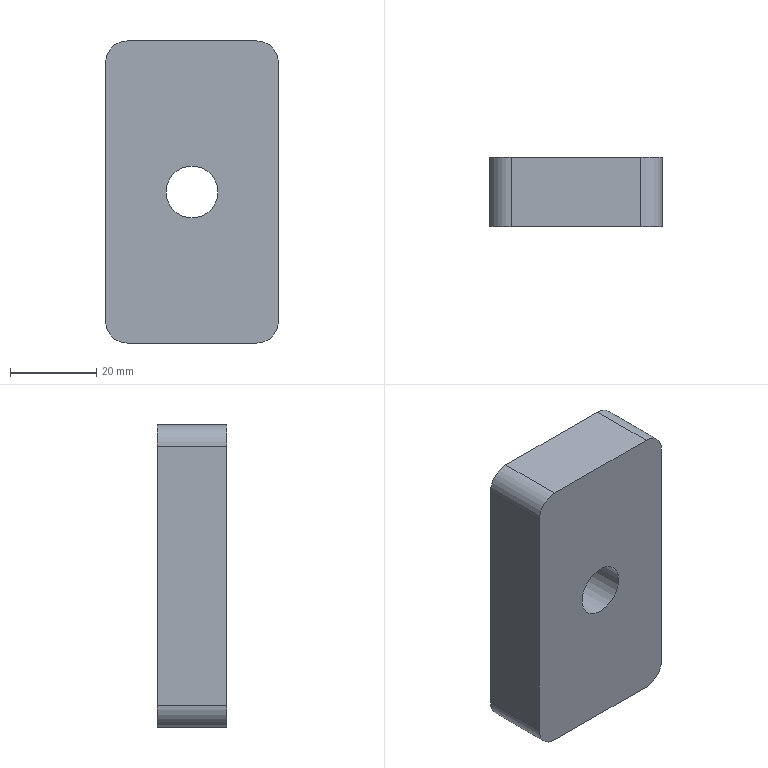Part | STEP file | HL4GZ-1.581.102 (tank fixing seat) | 1 solid | 11 faces | box 40 x 16 x 70 mm | volume 42647 mm3 | plane 6 | cylinder 5 | commonest cylinder face diameters 10 x4 12 x1
STEP:
#1=CARTESIAN_POINT('',(0.,0.,0.));
#2=DIRECTION('',(0.,0.,1.));
#3=DIRECTION('',(1.,0.,0.));
#4=AXIS2_PLACEMENT_3D('',#1,#2,#3);
#5=CARTESIAN_POINT('',(2027.,-666.,-40.));
#6=VERTEX_POINT('',#5);
#7=CARTESIAN_POINT('',(2022.,-666.,-45.));
#8=VERTEX_POINT('',#7);
#9=CARTESIAN_POINT('',(2027.,-666.,-45.));
#10=DIRECTION('',(0.,-1.,0.));
#11=DIRECTION('',(1.,0.,0.));
#12=AXIS2_PLACEMENT_3D('',#9,#10,#11);
#13=CIRCLE('',#12,5.);
#14=CARTESIAN_POINT('',(2027.,-662.,-45.));
#15=DIRECTION('',(0.,-1.,0.));
#16=DIRECTION('',(1.,0.,0.));
#17=AXIS2_PLACEMENT_3D('',#14,#15,#16);
#18=CYLINDRICAL_SURFACE('',#17,5.);
#19=CARTESIAN_POINT('',(0.,4.));
#20=DIRECTION('',(1.,0.));
#21=VECTOR('',#20,1.);
#22=LINE('',#19,#21);
#23=(GEOMETRIC_REPRESENTATION_CONTEXT(2)PARAMETRIC_REPRESENTATION_CONTEXT()REPRESENTATION_CONTEXT('',''));
#24=DEFINITIONAL_REPRESENTATION('',(#22),#23);
#25=PCURVE('',#18,#24);
#26=CARTESIAN_POINT('',(2021.,-666.,-75.));
#27=DIRECTION('',(0.,1.,0.));
#28=DIRECTION('',(1.,0.,0.));
#29=AXIS2_PLACEMENT_3D('',#26,#27,#28);
#30=PLANE('',#29);
#31=CARTESIAN_POINT('',(11.,-30.));
#32=CARTESIAN_POINT('',(11.,-38.66));
#33=CARTESIAN_POINT('',(3.5,-34.33));
#34=CARTESIAN_POINT('',(-4.,-30.));
#35=CARTESIAN_POINT('',(3.5,-25.67));
#36=CARTESIAN_POINT('',(11.,-21.34));
#37=CARTESIAN_POINT('',(11.,-30.));
#38=(BOUNDED_CURVE()B_SPLINE_CURVE(2,(#31,#32,#33,#34,#35,#36,#37),.UNSPECIFIED.,.T.,.F.)B_SPLINE_CURVE_WITH_KNOTS((1,2,2,2,2,1),(-2.094,0.,2.094,4.189,6.283,8.378),.UNSPECIFIED.)CURVE()GEOMETRIC_REPRESENTATION_ITEM()RATIONAL_B_SPLINE_CURVE((1.,0.5,1.,0.5,1.,0.5,1.))REPRESENTATION_ITEM(''));
#39=(GEOMETRIC_REPRESENTATION_CONTEXT(2)PARAMETRIC_REPRESENTATION_CONTEXT()REPRESENTATION_CONTEXT('',''));
#40=DEFINITIONAL_REPRESENTATION('',(#38),#39);
#41=PCURVE('',#30,#40);
#42=SURFACE_CURVE('',#13,(#25,#41),.PCURVE_S1.);
#43=EDGE_CURVE('',#6,#8,#42,.T.);
#44=ORIENTED_EDGE('',*,*,#43,.F.);
#45=CARTESIAN_POINT('',(2027.,-650.,-40.));
#46=VERTEX_POINT('',#45);
#47=CARTESIAN_POINT('',(2027.,-662.,-40.));
#48=DIRECTION('',(0.,-1.,0.));
#49=VECTOR('',#48,1.);
#50=LINE('',#47,#49);
#51=CARTESIAN_POINT('',(1.571,0.));
#52=DIRECTION('',(0.,1.));
#53=VECTOR('',#52,1.);
#54=LINE('',#51,#53);
#55=(GEOMETRIC_REPRESENTATION_CONTEXT(2)PARAMETRIC_REPRESENTATION_CONTEXT()REPRESENTATION_CONTEXT('',''));
#56=DEFINITIONAL_REPRESENTATION('',(#54),#55);
#57=PCURVE('',#18,#56);
#58=CARTESIAN_POINT('',(2062.,-662.,-40.));
#59=DIRECTION('',(0.,0.,-1.));
#60=DIRECTION('',(-1.,0.,0.));
#61=AXIS2_PLACEMENT_3D('',#58,#59,#60);
#62=PLANE('',#61);
#63=CARTESIAN_POINT('',(35.,0.));
#64=DIRECTION('',(0.,-1.));
#65=VECTOR('',#64,1.);
#66=LINE('',#63,#65);
#67=(GEOMETRIC_REPRESENTATION_CONTEXT(2)PARAMETRIC_REPRESENTATION_CONTEXT()REPRESENTATION_CONTEXT('',''));
#68=DEFINITIONAL_REPRESENTATION('',(#66),#67);
#69=PCURVE('',#62,#68);
#70=SURFACE_CURVE('',#50,(#57,#69),.PCURVE_S1.);
#71=EDGE_CURVE('',#46,#6,#70,.T.);
#72=ORIENTED_EDGE('',*,*,#71,.F.);
#73=CARTESIAN_POINT('',(2022.,-650.,-45.));
#74=VERTEX_POINT('',#73);
#75=CARTESIAN_POINT('',(2027.,-650.,-45.));
#76=DIRECTION('',(0.,1.,0.));
#77=DIRECTION('',(1.,0.,0.));
#78=AXIS2_PLACEMENT_3D('',#75,#76,#77);
#79=CIRCLE('',#78,5.);
#80=CARTESIAN_POINT('',(6.283,-12.));
#81=DIRECTION('',(-1.,0.));
#82=VECTOR('',#81,1.);
#83=LINE('',#80,#82);
#84=(GEOMETRIC_REPRESENTATION_CONTEXT(2)PARAMETRIC_REPRESENTATION_CONTEXT()REPRESENTATION_CONTEXT('',''));
#85=DEFINITIONAL_REPRESENTATION('',(#83),#84);
#86=PCURVE('',#18,#85);
#87=CARTESIAN_POINT('',(2021.,-650.,-75.));
#88=DIRECTION('',(0.,1.,0.));
#89=DIRECTION('',(1.,0.,0.));
#90=AXIS2_PLACEMENT_3D('',#87,#88,#89);
#91=PLANE('',#90);
#92=CARTESIAN_POINT('',(6.,-30.));
#93=DIRECTION('',(1.,0.));
#94=AXIS2_PLACEMENT_2D('',#92,#93);
#95=CIRCLE('',#94,5.);
#96=(GEOMETRIC_REPRESENTATION_CONTEXT(2)PARAMETRIC_REPRESENTATION_CONTEXT()REPRESENTATION_CONTEXT('',''));
#97=DEFINITIONAL_REPRESENTATION('',(#95),#96);
#98=PCURVE('',#91,#97);
#99=SURFACE_CURVE('',#79,(#86,#98),.PCURVE_S1.);
#100=EDGE_CURVE('',#74,#46,#99,.T.);
#101=ORIENTED_EDGE('',*,*,#100,.F.);
#102=CARTESIAN_POINT('',(2022.,-662.,-45.));
#103=DIRECTION('',(0.,1.,0.));
#104=VECTOR('',#103,1.);
#105=LINE('',#102,#104);
#106=CARTESIAN_POINT('',(3.142,0.));
#107=DIRECTION('',(0.,-1.));
#108=VECTOR('',#107,1.);
#109=LINE('',#106,#108);
#110=(GEOMETRIC_REPRESENTATION_CONTEXT(2)PARAMETRIC_REPRESENTATION_CONTEXT()REPRESENTATION_CONTEXT('',''));
#111=DEFINITIONAL_REPRESENTATION('',(#109),#110);
#112=PCURVE('',#18,#111);
#113=CARTESIAN_POINT('',(2022.,-662.,-75.));
#114=DIRECTION('',(-1.,0.,0.));
#115=DIRECTION('',(0.,0.,1.));
#116=AXIS2_PLACEMENT_3D('',#113,#114,#115);
#117=PLANE('',#116);
#118=CARTESIAN_POINT('',(30.,0.));
#119=DIRECTION('',(0.,1.));
#120=VECTOR('',#119,1.);
#121=LINE('',#118,#120);
#122=(GEOMETRIC_REPRESENTATION_CONTEXT(2)PARAMETRIC_REPRESENTATION_CONTEXT()REPRESENTATION_CONTEXT('',''));
#123=DEFINITIONAL_REPRESENTATION('',(#121),#122);
#124=PCURVE('',#117,#123);
#125=SURFACE_CURVE('',#105,(#112,#124),.PCURVE_S1.);
#126=EDGE_CURVE('',#8,#74,#125,.T.);
#127=ORIENTED_EDGE('',*,*,#126,.F.);
#128=EDGE_LOOP('',(#44,#72,#101,#127));
#129=FACE_BOUND('',#128,.T.);
#130=ADVANCED_FACE('',(#129),#18,.T.);
#131=CARTESIAN_POINT('',(2022.,-666.,-105.));
#132=VERTEX_POINT('',#131);
#133=CARTESIAN_POINT('',(2027.,-666.,-110.));
#134=VERTEX_POINT('',#133);
#135=CARTESIAN_POINT('',(2027.,-666.,-105.));
#136=DIRECTION('',(0.,-1.,0.));
#137=DIRECTION('',(1.,0.,0.));
#138=AXIS2_PLACEMENT_3D('',#135,#136,#137);
#139=CIRCLE('',#138,5.);
#140=CARTESIAN_POINT('',(2027.,-662.,-105.));
#141=DIRECTION('',(0.,-1.,0.));
#142=DIRECTION('',(1.,0.,0.));
#143=AXIS2_PLACEMENT_3D('',#140,#141,#142);
#144=CYLINDRICAL_SURFACE('',#143,5.);
#145=CARTESIAN_POINT('',(0.,4.));
#146=DIRECTION('',(1.,0.));
#147=VECTOR('',#146,1.);
#148=LINE('',#145,#147);
#149=(GEOMETRIC_REPRESENTATION_CONTEXT(2)PARAMETRIC_REPRESENTATION_CONTEXT()REPRESENTATION_CONTEXT('',''));
#150=DEFINITIONAL_REPRESENTATION('',(#148),#149);
#151=PCURVE('',#144,#150);
#152=CARTESIAN_POINT('',(11.,30.));
#153=CARTESIAN_POINT('',(11.,21.34));
#154=CARTESIAN_POINT('',(3.5,25.67));
#155=CARTESIAN_POINT('',(-4.,30.));
#156=CARTESIAN_POINT('',(3.5,34.33));
#157=CARTESIAN_POINT('',(11.,38.66));
#158=CARTESIAN_POINT('',(11.,30.));
#159=(BOUNDED_CURVE()B_SPLINE_CURVE(2,(#152,#153,#154,#155,#156,#157,#158),.UNSPECIFIED.,.T.,.F.)B_SPLINE_CURVE_WITH_KNOTS((1,2,2,2,2,1),(-2.094,0.,2.094,4.189,6.283,8.378),.UNSPECIFIED.)CURVE()GEOMETRIC_REPRESENTATION_ITEM()RATIONAL_B_SPLINE_CURVE((1.,0.5,1.,0.5,1.,0.5,1.))REPRESENTATION_ITEM(''));
#160=(GEOMETRIC_REPRESENTATION_CONTEXT(2)PARAMETRIC_REPRESENTATION_CONTEXT()REPRESENTATION_CONTEXT('',''));
#161=DEFINITIONAL_REPRESENTATION('',(#159),#160);
#162=PCURVE('',#30,#161);
#163=SURFACE_CURVE('',#139,(#151,#162),.PCURVE_S1.);
#164=EDGE_CURVE('',#132,#134,#163,.T.);
#165=ORIENTED_EDGE('',*,*,#164,.F.);
#166=CARTESIAN_POINT('',(2022.,-650.,-105.));
#167=VERTEX_POINT('',#166);
#168=CARTESIAN_POINT('',(2022.,-662.,-105.));
#169=DIRECTION('',(0.,-1.,0.));
#170=VECTOR('',#169,1.);
#171=LINE('',#168,#170);
#172=CARTESIAN_POINT('',(3.142,0.));
#173=DIRECTION('',(0.,1.));
#174=VECTOR('',#173,1.);
#175=LINE('',#172,#174);
#176=(GEOMETRIC_REPRESENTATION_CONTEXT(2)PARAMETRIC_REPRESENTATION_CONTEXT()REPRESENTATION_CONTEXT('',''));
#177=DEFINITIONAL_REPRESENTATION('',(#175),#176);
#178=PCURVE('',#144,#177);
#179=CARTESIAN_POINT('',(-30.,0.));
#180=DIRECTION('',(0.,-1.));
#181=VECTOR('',#180,1.);
#182=LINE('',#179,#181);
#183=(GEOMETRIC_REPRESENTATION_CONTEXT(2)PARAMETRIC_REPRESENTATION_CONTEXT()REPRESENTATION_CONTEXT('',''));
#184=DEFINITIONAL_REPRESENTATION('',(#182),#183);
#185=PCURVE('',#117,#184);
#186=SURFACE_CURVE('',#171,(#178,#185),.PCURVE_S1.);
#187=EDGE_CURVE('',#167,#132,#186,.T.);
#188=ORIENTED_EDGE('',*,*,#187,.F.);
#189=CARTESIAN_POINT('',(2027.,-650.,-110.));
#190=VERTEX_POINT('',#189);
#191=CARTESIAN_POINT('',(2027.,-650.,-105.));
#192=DIRECTION('',(0.,1.,0.));
#193=DIRECTION('',(1.,0.,0.));
#194=AXIS2_PLACEMENT_3D('',#191,#192,#193);
#195=CIRCLE('',#194,5.);
#196=CARTESIAN_POINT('',(6.283,-12.));
#197=DIRECTION('',(-1.,0.));
#198=VECTOR('',#197,1.);
#199=LINE('',#196,#198);
#200=(GEOMETRIC_REPRESENTATION_CONTEXT(2)PARAMETRIC_REPRESENTATION_CONTEXT()REPRESENTATION_CONTEXT('',''));
#201=DEFINITIONAL_REPRESENTATION('',(#199),#200);
#202=PCURVE('',#144,#201);
#203=CARTESIAN_POINT('',(6.,30.));
#204=DIRECTION('',(1.,0.));
#205=AXIS2_PLACEMENT_2D('',#203,#204);
#206=CIRCLE('',#205,5.);
#207=(GEOMETRIC_REPRESENTATION_CONTEXT(2)PARAMETRIC_REPRESENTATION_CONTEXT()REPRESENTATION_CONTEXT('',''));
#208=DEFINITIONAL_REPRESENTATION('',(#206),#207);
#209=PCURVE('',#91,#208);
#210=SURFACE_CURVE('',#195,(#202,#209),.PCURVE_S1.);
#211=EDGE_CURVE('',#190,#167,#210,.T.);
#212=ORIENTED_EDGE('',*,*,#211,.F.);
#213=CARTESIAN_POINT('',(2027.,-662.,-110.));
#214=DIRECTION('',(0.,1.,0.));
#215=VECTOR('',#214,1.);
#216=LINE('',#213,#215);
#217=CARTESIAN_POINT('',(4.712,0.));
#218=DIRECTION('',(0.,-1.));
#219=VECTOR('',#218,1.);
#220=LINE('',#217,#219);
#221=(GEOMETRIC_REPRESENTATION_CONTEXT(2)PARAMETRIC_REPRESENTATION_CONTEXT()REPRESENTATION_CONTEXT('',''));
#222=DEFINITIONAL_REPRESENTATION('',(#220),#221);
#223=PCURVE('',#144,#222);
#224=CARTESIAN_POINT('',(2062.,-662.,-110.));
#225=DIRECTION('',(0.,0.,1.));
#226=DIRECTION('',(1.,0.,0.));
#227=AXIS2_PLACEMENT_3D('',#224,#225,#226);
#228=PLANE('',#227);
#229=CARTESIAN_POINT('',(-35.,0.));
#230=DIRECTION('',(0.,1.));
#231=VECTOR('',#230,1.);
#232=LINE('',#229,#231);
#233=(GEOMETRIC_REPRESENTATION_CONTEXT(2)PARAMETRIC_REPRESENTATION_CONTEXT()REPRESENTATION_CONTEXT('',''));
#234=DEFINITIONAL_REPRESENTATION('',(#232),#233);
#235=PCURVE('',#228,#234);
#236=SURFACE_CURVE('',#216,(#223,#235),.PCURVE_S1.);
#237=EDGE_CURVE('',#134,#190,#236,.T.);
#238=ORIENTED_EDGE('',*,*,#237,.F.);
#239=EDGE_LOOP('',(#165,#188,#212,#238));
#240=FACE_BOUND('',#239,.T.);
#241=ADVANCED_FACE('',(#240),#144,.T.);
#242=CARTESIAN_POINT('',(2062.,-666.,-45.));
#243=VERTEX_POINT('',#242);
#244=CARTESIAN_POINT('',(2057.,-666.,-40.));
#245=VERTEX_POINT('',#244);
#246=CARTESIAN_POINT('',(2057.,-666.,-45.));
#247=DIRECTION('',(0.,-1.,0.));
#248=DIRECTION('',(1.,0.,0.));
#249=AXIS2_PLACEMENT_3D('',#246,#247,#248);
#250=CIRCLE('',#249,5.);
#251=CARTESIAN_POINT('',(2057.,-662.,-45.));
#252=DIRECTION('',(0.,-1.,0.));
#253=DIRECTION('',(1.,0.,0.));
#254=AXIS2_PLACEMENT_3D('',#251,#252,#253);
#255=CYLINDRICAL_SURFACE('',#254,5.);
#256=CARTESIAN_POINT('',(0.,4.));
#257=DIRECTION('',(1.,0.));
#258=VECTOR('',#257,1.);
#259=LINE('',#256,#258);
#260=(GEOMETRIC_REPRESENTATION_CONTEXT(2)PARAMETRIC_REPRESENTATION_CONTEXT()REPRESENTATION_CONTEXT('',''));
#261=DEFINITIONAL_REPRESENTATION('',(#259),#260);
#262=PCURVE('',#255,#261);
#263=CARTESIAN_POINT('',(41.,-30.));
#264=CARTESIAN_POINT('',(41.,-38.66));
#265=CARTESIAN_POINT('',(33.5,-34.33));
#266=CARTESIAN_POINT('',(26.,-30.));
#267=CARTESIAN_POINT('',(33.5,-25.67));
#268=CARTESIAN_POINT('',(41.,-21.34));
#269=CARTESIAN_POINT('',(41.,-30.));
#270=(BOUNDED_CURVE()B_SPLINE_CURVE(2,(#263,#264,#265,#266,#267,#268,#269),.UNSPECIFIED.,.T.,.F.)B_SPLINE_CURVE_WITH_KNOTS((1,2,2,2,2,1),(-2.094,0.,2.094,4.189,6.283,8.378),.UNSPECIFIED.)CURVE()GEOMETRIC_REPRESENTATION_ITEM()RATIONAL_B_SPLINE_CURVE((1.,0.5,1.,0.5,1.,0.5,1.))REPRESENTATION_ITEM(''));
#271=(GEOMETRIC_REPRESENTATION_CONTEXT(2)PARAMETRIC_REPRESENTATION_CONTEXT()REPRESENTATION_CONTEXT('',''));
#272=DEFINITIONAL_REPRESENTATION('',(#270),#271);
#273=PCURVE('',#30,#272);
#274=SURFACE_CURVE('',#250,(#262,#273),.PCURVE_S1.);
#275=EDGE_CURVE('',#243,#245,#274,.T.);
#276=ORIENTED_EDGE('',*,*,#275,.F.);
#277=CARTESIAN_POINT('',(2062.,-650.,-45.));
#278=VERTEX_POINT('',#277);
#279=CARTESIAN_POINT('',(2062.,-662.,-45.));
#280=DIRECTION('',(0.,-1.,0.));
#281=VECTOR('',#280,1.);
#282=LINE('',#279,#281);
#283=CARTESIAN_POINT('',(0.,0.));
#284=DIRECTION('',(0.,1.));
#285=VECTOR('',#284,1.);
#286=LINE('',#283,#285);
#287=(GEOMETRIC_REPRESENTATION_CONTEXT(2)PARAMETRIC_REPRESENTATION_CONTEXT()REPRESENTATION_CONTEXT('',''));
#288=DEFINITIONAL_REPRESENTATION('',(#286),#287);
#289=PCURVE('',#255,#288);
#290=CARTESIAN_POINT('',(2062.,-662.,-75.));
#291=DIRECTION('',(1.,0.,0.));
#292=DIRECTION('',(0.,0.,-1.));
#293=AXIS2_PLACEMENT_3D('',#290,#291,#292);
#294=PLANE('',#293);
#295=CARTESIAN_POINT('',(-30.,0.));
#296=DIRECTION('',(0.,-1.));
#297=VECTOR('',#296,1.);
#298=LINE('',#295,#297);
#299=(GEOMETRIC_REPRESENTATION_CONTEXT(2)PARAMETRIC_REPRESENTATION_CONTEXT()REPRESENTATION_CONTEXT('',''));
#300=DEFINITIONAL_REPRESENTATION('',(#298),#299);
#301=PCURVE('',#294,#300);
#302=SURFACE_CURVE('',#282,(#289,#301),.PCURVE_S1.);
#303=EDGE_CURVE('',#278,#243,#302,.T.);
#304=ORIENTED_EDGE('',*,*,#303,.F.);
#305=CARTESIAN_POINT('',(2057.,-650.,-40.));
#306=VERTEX_POINT('',#305);
#307=CARTESIAN_POINT('',(2057.,-650.,-45.));
#308=DIRECTION('',(0.,1.,0.));
#309=DIRECTION('',(1.,0.,0.));
#310=AXIS2_PLACEMENT_3D('',#307,#308,#309);
#311=CIRCLE('',#310,5.);
#312=CARTESIAN_POINT('',(6.283,-12.));
#313=DIRECTION('',(-1.,0.));
#314=VECTOR('',#313,1.);
#315=LINE('',#312,#314);
#316=(GEOMETRIC_REPRESENTATION_CONTEXT(2)PARAMETRIC_REPRESENTATION_CONTEXT()REPRESENTATION_CONTEXT('',''));
#317=DEFINITIONAL_REPRESENTATION('',(#315),#316);
#318=PCURVE('',#255,#317);
#319=CARTESIAN_POINT('',(36.,-30.));
#320=DIRECTION('',(1.,0.));
#321=AXIS2_PLACEMENT_2D('',#319,#320);
#322=CIRCLE('',#321,5.);
#323=(GEOMETRIC_REPRESENTATION_CONTEXT(2)PARAMETRIC_REPRESENTATION_CONTEXT()REPRESENTATION_CONTEXT('',''));
#324=DEFINITIONAL_REPRESENTATION('',(#322),#323);
#325=PCURVE('',#91,#324);
#326=SURFACE_CURVE('',#311,(#318,#325),.PCURVE_S1.);
#327=EDGE_CURVE('',#306,#278,#326,.T.);
#328=ORIENTED_EDGE('',*,*,#327,.F.);
#329=CARTESIAN_POINT('',(2057.,-662.,-40.));
#330=DIRECTION('',(0.,1.,0.));
#331=VECTOR('',#330,1.);
#332=LINE('',#329,#331);
#333=CARTESIAN_POINT('',(1.571,0.));
#334=DIRECTION('',(0.,-1.));
#335=VECTOR('',#334,1.);
#336=LINE('',#333,#335);
#337=(GEOMETRIC_REPRESENTATION_CONTEXT(2)PARAMETRIC_REPRESENTATION_CONTEXT()REPRESENTATION_CONTEXT('',''));
#338=DEFINITIONAL_REPRESENTATION('',(#336),#337);
#339=PCURVE('',#255,#338);
#340=CARTESIAN_POINT('',(5.,0.));
#341=DIRECTION('',(0.,1.));
#342=VECTOR('',#341,1.);
#343=LINE('',#340,#342);
#344=(GEOMETRIC_REPRESENTATION_CONTEXT(2)PARAMETRIC_REPRESENTATION_CONTEXT()REPRESENTATION_CONTEXT('',''));
#345=DEFINITIONAL_REPRESENTATION('',(#343),#344);
#346=PCURVE('',#62,#345);
#347=SURFACE_CURVE('',#332,(#339,#346),.PCURVE_S1.);
#348=EDGE_CURVE('',#245,#306,#347,.T.);
#349=ORIENTED_EDGE('',*,*,#348,.F.);
#350=EDGE_LOOP('',(#276,#304,#328,#349));
#351=FACE_BOUND('',#350,.T.);
#352=ADVANCED_FACE('',(#351),#255,.T.);
#353=CARTESIAN_POINT('',(2057.,-666.,-110.));
#354=VERTEX_POINT('',#353);
#355=CARTESIAN_POINT('',(2062.,-666.,-105.));
#356=VERTEX_POINT('',#355);
#357=CARTESIAN_POINT('',(2057.,-666.,-105.));
#358=DIRECTION('',(0.,-1.,0.));
#359=DIRECTION('',(1.,0.,0.));
#360=AXIS2_PLACEMENT_3D('',#357,#358,#359);
#361=CIRCLE('',#360,5.);
#362=CARTESIAN_POINT('',(2057.,-662.,-105.));
#363=DIRECTION('',(0.,1.,0.));
#364=DIRECTION('',(-1.,0.,0.));
#365=AXIS2_PLACEMENT_3D('',#362,#363,#364);
#366=CYLINDRICAL_SURFACE('',#365,5.);
#367=CARTESIAN_POINT('',(9.425,-4.));
#368=DIRECTION('',(-1.,0.));
#369=VECTOR('',#368,1.);
#370=LINE('',#367,#369);
#371=(GEOMETRIC_REPRESENTATION_CONTEXT(2)PARAMETRIC_REPRESENTATION_CONTEXT()REPRESENTATION_CONTEXT('',''));
#372=DEFINITIONAL_REPRESENTATION('',(#370),#371);
#373=PCURVE('',#366,#372);
#374=CARTESIAN_POINT('',(41.,30.));
#375=CARTESIAN_POINT('',(41.,21.34));
#376=CARTESIAN_POINT('',(33.5,25.67));
#377=CARTESIAN_POINT('',(26.,30.));
#378=CARTESIAN_POINT('',(33.5,34.33));
#379=CARTESIAN_POINT('',(41.,38.66));
#380=CARTESIAN_POINT('',(41.,30.));
#381=(BOUNDED_CURVE()B_SPLINE_CURVE(2,(#374,#375,#376,#377,#378,#379,#380),.UNSPECIFIED.,.T.,.F.)B_SPLINE_CURVE_WITH_KNOTS((1,2,2,2,2,1),(-2.094,0.,2.094,4.189,6.283,8.378),.UNSPECIFIED.)CURVE()GEOMETRIC_REPRESENTATION_ITEM()RATIONAL_B_SPLINE_CURVE((1.,0.5,1.,0.5,1.,0.5,1.))REPRESENTATION_ITEM(''));
#382=(GEOMETRIC_REPRESENTATION_CONTEXT(2)PARAMETRIC_REPRESENTATION_CONTEXT()REPRESENTATION_CONTEXT('',''));
#383=DEFINITIONAL_REPRESENTATION('',(#381),#382);
#384=PCURVE('',#30,#383);
#385=SURFACE_CURVE('',#361,(#373,#384),.PCURVE_S1.);
#386=EDGE_CURVE('',#354,#356,#385,.T.);
#387=ORIENTED_EDGE('',*,*,#386,.F.);
#388=CARTESIAN_POINT('',(2057.,-650.,-110.));
#389=VERTEX_POINT('',#388);
#390=CARTESIAN_POINT('',(2057.,-662.,-110.));
#391=DIRECTION('',(0.,-1.,0.));
#392=VECTOR('',#391,1.);
#393=LINE('',#390,#392);
#394=CARTESIAN_POINT('',(4.712,0.));
#395=DIRECTION('',(0.,-1.));
#396=VECTOR('',#395,1.);
#397=LINE('',#394,#396);
#398=(GEOMETRIC_REPRESENTATION_CONTEXT(2)PARAMETRIC_REPRESENTATION_CONTEXT()REPRESENTATION_CONTEXT('',''));
#399=DEFINITIONAL_REPRESENTATION('',(#397),#398);
#400=PCURVE('',#366,#399);
#401=CARTESIAN_POINT('',(-5.,0.));
#402=DIRECTION('',(0.,-1.));
#403=VECTOR('',#402,1.);
#404=LINE('',#401,#403);
#405=(GEOMETRIC_REPRESENTATION_CONTEXT(2)PARAMETRIC_REPRESENTATION_CONTEXT()REPRESENTATION_CONTEXT('',''));
#406=DEFINITIONAL_REPRESENTATION('',(#404),#405);
#407=PCURVE('',#228,#406);
#408=SURFACE_CURVE('',#393,(#400,#407),.PCURVE_S1.);
#409=EDGE_CURVE('',#389,#354,#408,.T.);
#410=ORIENTED_EDGE('',*,*,#409,.F.);
#411=CARTESIAN_POINT('',(2062.,-650.,-105.));
#412=VERTEX_POINT('',#411);
#413=CARTESIAN_POINT('',(2057.,-650.,-105.));
#414=DIRECTION('',(0.,1.,0.));
#415=DIRECTION('',(1.,0.,0.));
#416=AXIS2_PLACEMENT_3D('',#413,#414,#415);
#417=CIRCLE('',#416,5.);
#418=CARTESIAN_POINT('',(3.142,12.));
#419=DIRECTION('',(1.,0.));
#420=VECTOR('',#419,1.);
#421=LINE('',#418,#420);
#422=(GEOMETRIC_REPRESENTATION_CONTEXT(2)PARAMETRIC_REPRESENTATION_CONTEXT()REPRESENTATION_CONTEXT('',''));
#423=DEFINITIONAL_REPRESENTATION('',(#421),#422);
#424=PCURVE('',#366,#423);
#425=CARTESIAN_POINT('',(36.,30.));
#426=DIRECTION('',(1.,0.));
#427=AXIS2_PLACEMENT_2D('',#425,#426);
#428=CIRCLE('',#427,5.);
#429=(GEOMETRIC_REPRESENTATION_CONTEXT(2)PARAMETRIC_REPRESENTATION_CONTEXT()REPRESENTATION_CONTEXT('',''));
#430=DEFINITIONAL_REPRESENTATION('',(#428),#429);
#431=PCURVE('',#91,#430);
#432=SURFACE_CURVE('',#417,(#424,#431),.PCURVE_S1.);
#433=EDGE_CURVE('',#412,#389,#432,.T.);
#434=ORIENTED_EDGE('',*,*,#433,.F.);
#435=CARTESIAN_POINT('',(2062.,-662.,-105.));
#436=DIRECTION('',(0.,1.,0.));
#437=VECTOR('',#436,1.);
#438=LINE('',#435,#437);
#439=CARTESIAN_POINT('',(3.142,0.));
#440=DIRECTION('',(0.,1.));
#441=VECTOR('',#440,1.);
#442=LINE('',#439,#441);
#443=(GEOMETRIC_REPRESENTATION_CONTEXT(2)PARAMETRIC_REPRESENTATION_CONTEXT()REPRESENTATION_CONTEXT('',''));
#444=DEFINITIONAL_REPRESENTATION('',(#442),#443);
#445=PCURVE('',#366,#444);
#446=CARTESIAN_POINT('',(30.,0.));
#447=DIRECTION('',(0.,1.));
#448=VECTOR('',#447,1.);
#449=LINE('',#446,#448);
#450=(GEOMETRIC_REPRESENTATION_CONTEXT(2)PARAMETRIC_REPRESENTATION_CONTEXT()REPRESENTATION_CONTEXT('',''));
#451=DEFINITIONAL_REPRESENTATION('',(#449),#450);
#452=PCURVE('',#294,#451);
#453=SURFACE_CURVE('',#438,(#445,#452),.PCURVE_S1.);
#454=EDGE_CURVE('',#356,#412,#453,.T.);
#455=ORIENTED_EDGE('',*,*,#454,.F.);
#456=EDGE_LOOP('',(#387,#410,#434,#455));
#457=FACE_BOUND('',#456,.T.);
#458=ADVANCED_FACE('',(#457),#366,.T.);
#459=CARTESIAN_POINT('',(2048.,-666.,-75.));
#460=VERTEX_POINT('',#459);
#461=CARTESIAN_POINT('',(2042.,-666.,-75.));
#462=DIRECTION('',(0.,-1.,0.));
#463=DIRECTION('',(1.,0.,0.));
#464=AXIS2_PLACEMENT_3D('',#461,#462,#463);
#465=CIRCLE('',#464,6.);
#466=CARTESIAN_POINT('',(27.,0.));
#467=CARTESIAN_POINT('',(27.,-10.392));
#468=CARTESIAN_POINT('',(18.,-5.196));
#469=CARTESIAN_POINT('',(9.,0.));
#470=CARTESIAN_POINT('',(18.,5.196));
#471=CARTESIAN_POINT('',(27.,10.392));
#472=CARTESIAN_POINT('',(27.,0.));
#473=(BOUNDED_CURVE()B_SPLINE_CURVE(2,(#466,#467,#468,#469,#470,#471,#472),.UNSPECIFIED.,.T.,.F.)B_SPLINE_CURVE_WITH_KNOTS((1,2,2,2,2,1),(-2.094,0.,2.094,4.189,6.283,8.378),.UNSPECIFIED.)CURVE()GEOMETRIC_REPRESENTATION_ITEM()RATIONAL_B_SPLINE_CURVE((1.,0.5,1.,0.5,1.,0.5,1.))REPRESENTATION_ITEM(''));
#474=(GEOMETRIC_REPRESENTATION_CONTEXT(2)PARAMETRIC_REPRESENTATION_CONTEXT()REPRESENTATION_CONTEXT('',''));
#475=DEFINITIONAL_REPRESENTATION('',(#473),#474);
#476=PCURVE('',#30,#475);
#477=CARTESIAN_POINT('',(2042.,-662.,-75.));
#478=DIRECTION('',(0.,-1.,0.));
#479=DIRECTION('',(1.,0.,0.));
#480=AXIS2_PLACEMENT_3D('',#477,#478,#479);
#481=CYLINDRICAL_SURFACE('',#480,6.);
#482=CARTESIAN_POINT('',(0.,4.));
#483=DIRECTION('',(1.,0.));
#484=VECTOR('',#483,1.);
#485=LINE('',#482,#484);
#486=(GEOMETRIC_REPRESENTATION_CONTEXT(2)PARAMETRIC_REPRESENTATION_CONTEXT()REPRESENTATION_CONTEXT('',''));
#487=DEFINITIONAL_REPRESENTATION('',(#485),#486);
#488=PCURVE('',#481,#487);
#489=SURFACE_CURVE('',#465,(#476,#488),.PCURVE_S1.);
#490=EDGE_CURVE('',#460,#460,#489,.T.);
#491=ORIENTED_EDGE('',*,*,#490,.F.);
#492=EDGE_LOOP('',(#491));
#493=FACE_BOUND('',#492,.T.);
#494=CARTESIAN_POINT('',(2022.,-666.,-75.));
#495=DIRECTION('',(0.,0.,1.));
#496=VECTOR('',#495,1.);
#497=LINE('',#494,#496);
#498=CARTESIAN_POINT('',(1.,0.));
#499=DIRECTION('',(0.,-1.));
#500=VECTOR('',#499,1.);
#501=LINE('',#498,#500);
#502=(GEOMETRIC_REPRESENTATION_CONTEXT(2)PARAMETRIC_REPRESENTATION_CONTEXT()REPRESENTATION_CONTEXT('',''));
#503=DEFINITIONAL_REPRESENTATION('',(#501),#502);
#504=PCURVE('',#30,#503);
#505=CARTESIAN_POINT('',(0.,-4.));
#506=DIRECTION('',(1.,0.));
#507=VECTOR('',#506,1.);
#508=LINE('',#505,#507);
#509=(GEOMETRIC_REPRESENTATION_CONTEXT(2)PARAMETRIC_REPRESENTATION_CONTEXT()REPRESENTATION_CONTEXT('',''));
#510=DEFINITIONAL_REPRESENTATION('',(#508),#509);
#511=PCURVE('',#117,#510);
#512=SURFACE_CURVE('',#497,(#504,#511),.PCURVE_S1.);
#513=EDGE_CURVE('',#132,#8,#512,.T.);
#514=ORIENTED_EDGE('',*,*,#513,.F.);
#515=ORIENTED_EDGE('',*,*,#164,.T.);
#516=CARTESIAN_POINT('',(2062.,-666.,-110.));
#517=DIRECTION('',(1.,0.,0.));
#518=VECTOR('',#517,1.);
#519=LINE('',#516,#518);
#520=CARTESIAN_POINT('',(41.,35.));
#521=DIRECTION('',(1.,0.));
#522=VECTOR('',#521,1.);
#523=LINE('',#520,#522);
#524=(GEOMETRIC_REPRESENTATION_CONTEXT(2)PARAMETRIC_REPRESENTATION_CONTEXT()REPRESENTATION_CONTEXT('',''));
#525=DEFINITIONAL_REPRESENTATION('',(#523),#524);
#526=PCURVE('',#30,#525);
#527=CARTESIAN_POINT('',(0.,-4.));
#528=DIRECTION('',(1.,0.));
#529=VECTOR('',#528,1.);
#530=LINE('',#527,#529);
#531=(GEOMETRIC_REPRESENTATION_CONTEXT(2)PARAMETRIC_REPRESENTATION_CONTEXT()REPRESENTATION_CONTEXT('',''));
#532=DEFINITIONAL_REPRESENTATION('',(#530),#531);
#533=PCURVE('',#228,#532);
#534=SURFACE_CURVE('',#519,(#526,#533),.PCURVE_S1.);
#535=EDGE_CURVE('',#134,#354,#534,.T.);
#536=ORIENTED_EDGE('',*,*,#535,.T.);
#537=ORIENTED_EDGE('',*,*,#386,.T.);
#538=CARTESIAN_POINT('',(2062.,-666.,-75.));
#539=DIRECTION('',(0.,0.,-1.));
#540=VECTOR('',#539,1.);
#541=LINE('',#538,#540);
#542=CARTESIAN_POINT('',(41.,0.));
#543=DIRECTION('',(0.,1.));
#544=VECTOR('',#543,1.);
#545=LINE('',#542,#544);
#546=(GEOMETRIC_REPRESENTATION_CONTEXT(2)PARAMETRIC_REPRESENTATION_CONTEXT()REPRESENTATION_CONTEXT('',''));
#547=DEFINITIONAL_REPRESENTATION('',(#545),#546);
#548=PCURVE('',#30,#547);
#549=CARTESIAN_POINT('',(0.,-4.));
#550=DIRECTION('',(1.,0.));
#551=VECTOR('',#550,1.);
#552=LINE('',#549,#551);
#553=(GEOMETRIC_REPRESENTATION_CONTEXT(2)PARAMETRIC_REPRESENTATION_CONTEXT()REPRESENTATION_CONTEXT('',''));
#554=DEFINITIONAL_REPRESENTATION('',(#552),#553);
#555=PCURVE('',#294,#554);
#556=SURFACE_CURVE('',#541,(#548,#555),.PCURVE_S1.);
#557=EDGE_CURVE('',#243,#356,#556,.T.);
#558=ORIENTED_EDGE('',*,*,#557,.F.);
#559=ORIENTED_EDGE('',*,*,#275,.T.);
#560=CARTESIAN_POINT('',(2062.,-666.,-40.));
#561=DIRECTION('',(-1.,0.,0.));
#562=VECTOR('',#561,1.);
#563=LINE('',#560,#562);
#564=CARTESIAN_POINT('',(41.,-35.));
#565=DIRECTION('',(-1.,0.));
#566=VECTOR('',#565,1.);
#567=LINE('',#564,#566);
#568=(GEOMETRIC_REPRESENTATION_CONTEXT(2)PARAMETRIC_REPRESENTATION_CONTEXT()REPRESENTATION_CONTEXT('',''));
#569=DEFINITIONAL_REPRESENTATION('',(#567),#568);
#570=PCURVE('',#30,#569);
#571=CARTESIAN_POINT('',(0.,-4.));
#572=DIRECTION('',(1.,0.));
#573=VECTOR('',#572,1.);
#574=LINE('',#571,#573);
#575=(GEOMETRIC_REPRESENTATION_CONTEXT(2)PARAMETRIC_REPRESENTATION_CONTEXT()REPRESENTATION_CONTEXT('',''));
#576=DEFINITIONAL_REPRESENTATION('',(#574),#575);
#577=PCURVE('',#62,#576);
#578=SURFACE_CURVE('',#563,(#570,#577),.PCURVE_S1.);
#579=EDGE_CURVE('',#245,#6,#578,.T.);
#580=ORIENTED_EDGE('',*,*,#579,.T.);
#581=ORIENTED_EDGE('',*,*,#43,.T.);
#582=EDGE_LOOP('',(#514,#515,#536,#537,#558,#559,#580,#581));
#583=FACE_BOUND('',#582,.T.);
#584=ADVANCED_FACE('',(#493,#583),#30,.F.);
#585=CARTESIAN_POINT('',(2048.,-650.,-75.));
#586=VERTEX_POINT('',#585);
#587=CARTESIAN_POINT('',(2042.,-650.,-75.));
#588=DIRECTION('',(0.,-1.,0.));
#589=DIRECTION('',(1.,0.,0.));
#590=AXIS2_PLACEMENT_3D('',#587,#588,#589);
#591=CIRCLE('',#590,6.);
#592=CARTESIAN_POINT('',(27.,0.));
#593=CARTESIAN_POINT('',(27.,-10.392));
#594=CARTESIAN_POINT('',(18.,-5.196));
#595=CARTESIAN_POINT('',(9.,0.));
#596=CARTESIAN_POINT('',(18.,5.196));
#597=CARTESIAN_POINT('',(27.,10.392));
#598=CARTESIAN_POINT('',(27.,0.));
#599=(BOUNDED_CURVE()B_SPLINE_CURVE(2,(#592,#593,#594,#595,#596,#597,#598),.UNSPECIFIED.,.T.,.F.)B_SPLINE_CURVE_WITH_KNOTS((1,2,2,2,2,1),(-2.094,0.,2.094,4.189,6.283,8.378),.UNSPECIFIED.)CURVE()GEOMETRIC_REPRESENTATION_ITEM()RATIONAL_B_SPLINE_CURVE((1.,0.5,1.,0.5,1.,0.5,1.))REPRESENTATION_ITEM(''));
#600=(GEOMETRIC_REPRESENTATION_CONTEXT(2)PARAMETRIC_REPRESENTATION_CONTEXT()REPRESENTATION_CONTEXT('',''));
#601=DEFINITIONAL_REPRESENTATION('',(#599),#600);
#602=PCURVE('',#91,#601);
#603=CARTESIAN_POINT('',(0.,-12.));
#604=DIRECTION('',(1.,0.));
#605=VECTOR('',#604,1.);
#606=LINE('',#603,#605);
#607=(GEOMETRIC_REPRESENTATION_CONTEXT(2)PARAMETRIC_REPRESENTATION_CONTEXT()REPRESENTATION_CONTEXT('',''));
#608=DEFINITIONAL_REPRESENTATION('',(#606),#607);
#609=PCURVE('',#481,#608);
#610=SURFACE_CURVE('',#591,(#602,#609),.PCURVE_S1.);
#611=EDGE_CURVE('',#586,#586,#610,.T.);
#612=ORIENTED_EDGE('',*,*,#611,.T.);
#613=EDGE_LOOP('',(#612));
#614=FACE_BOUND('',#613,.T.);
#615=CARTESIAN_POINT('',(2021.,-650.,-40.));
#616=DIRECTION('',(-1.,0.,0.));
#617=VECTOR('',#616,1.);
#618=LINE('',#615,#617);
#619=CARTESIAN_POINT('',(0.,-35.));
#620=DIRECTION('',(-1.,0.));
#621=VECTOR('',#620,1.);
#622=LINE('',#619,#621);
#623=(GEOMETRIC_REPRESENTATION_CONTEXT(2)PARAMETRIC_REPRESENTATION_CONTEXT()REPRESENTATION_CONTEXT('',''));
#624=DEFINITIONAL_REPRESENTATION('',(#622),#623);
#625=PCURVE('',#91,#624);
#626=CARTESIAN_POINT('',(41.,12.));
#627=DIRECTION('',(1.,0.));
#628=VECTOR('',#627,1.);
#629=LINE('',#626,#628);
#630=(GEOMETRIC_REPRESENTATION_CONTEXT(2)PARAMETRIC_REPRESENTATION_CONTEXT()REPRESENTATION_CONTEXT('',''));
#631=DEFINITIONAL_REPRESENTATION('',(#629),#630);
#632=PCURVE('',#62,#631);
#633=SURFACE_CURVE('',#618,(#625,#632),.PCURVE_S1.);
#634=EDGE_CURVE('',#306,#46,#633,.T.);
#635=ORIENTED_EDGE('',*,*,#634,.F.);
#636=ORIENTED_EDGE('',*,*,#327,.T.);
#637=CARTESIAN_POINT('',(2062.,-650.,-75.));
#638=DIRECTION('',(0.,0.,-1.));
#639=VECTOR('',#638,1.);
#640=LINE('',#637,#639);
#641=CARTESIAN_POINT('',(41.,0.));
#642=DIRECTION('',(0.,1.));
#643=VECTOR('',#642,1.);
#644=LINE('',#641,#643);
#645=(GEOMETRIC_REPRESENTATION_CONTEXT(2)PARAMETRIC_REPRESENTATION_CONTEXT()REPRESENTATION_CONTEXT('',''));
#646=DEFINITIONAL_REPRESENTATION('',(#644),#645);
#647=PCURVE('',#91,#646);
#648=CARTESIAN_POINT('',(0.,12.));
#649=DIRECTION('',(1.,0.));
#650=VECTOR('',#649,1.);
#651=LINE('',#648,#650);
#652=(GEOMETRIC_REPRESENTATION_CONTEXT(2)PARAMETRIC_REPRESENTATION_CONTEXT()REPRESENTATION_CONTEXT('',''));
#653=DEFINITIONAL_REPRESENTATION('',(#651),#652);
#654=PCURVE('',#294,#653);
#655=SURFACE_CURVE('',#640,(#647,#654),.PCURVE_S1.);
#656=EDGE_CURVE('',#278,#412,#655,.T.);
#657=ORIENTED_EDGE('',*,*,#656,.T.);
#658=ORIENTED_EDGE('',*,*,#433,.T.);
#659=CARTESIAN_POINT('',(2021.,-650.,-110.));
#660=DIRECTION('',(1.,0.,0.));
#661=VECTOR('',#660,1.);
#662=LINE('',#659,#661);
#663=CARTESIAN_POINT('',(0.,35.));
#664=DIRECTION('',(1.,0.));
#665=VECTOR('',#664,1.);
#666=LINE('',#663,#665);
#667=(GEOMETRIC_REPRESENTATION_CONTEXT(2)PARAMETRIC_REPRESENTATION_CONTEXT()REPRESENTATION_CONTEXT('',''));
#668=DEFINITIONAL_REPRESENTATION('',(#666),#667);
#669=PCURVE('',#91,#668);
#670=CARTESIAN_POINT('',(-41.,12.));
#671=DIRECTION('',(1.,0.));
#672=VECTOR('',#671,1.);
#673=LINE('',#670,#672);
#674=(GEOMETRIC_REPRESENTATION_CONTEXT(2)PARAMETRIC_REPRESENTATION_CONTEXT()REPRESENTATION_CONTEXT('',''));
#675=DEFINITIONAL_REPRESENTATION('',(#673),#674);
#676=PCURVE('',#228,#675);
#677=SURFACE_CURVE('',#662,(#669,#676),.PCURVE_S1.);
#678=EDGE_CURVE('',#190,#389,#677,.T.);
#679=ORIENTED_EDGE('',*,*,#678,.F.);
#680=ORIENTED_EDGE('',*,*,#211,.T.);
#681=CARTESIAN_POINT('',(2022.,-650.,-75.));
#682=DIRECTION('',(0.,0.,1.));
#683=VECTOR('',#682,1.);
#684=LINE('',#681,#683);
#685=CARTESIAN_POINT('',(1.,0.));
#686=DIRECTION('',(0.,-1.));
#687=VECTOR('',#686,1.);
#688=LINE('',#685,#687);
#689=(GEOMETRIC_REPRESENTATION_CONTEXT(2)PARAMETRIC_REPRESENTATION_CONTEXT()REPRESENTATION_CONTEXT('',''));
#690=DEFINITIONAL_REPRESENTATION('',(#688),#689);
#691=PCURVE('',#91,#690);
#692=CARTESIAN_POINT('',(0.,12.));
#693=DIRECTION('',(1.,0.));
#694=VECTOR('',#693,1.);
#695=LINE('',#692,#694);
#696=(GEOMETRIC_REPRESENTATION_CONTEXT(2)PARAMETRIC_REPRESENTATION_CONTEXT()REPRESENTATION_CONTEXT('',''));
#697=DEFINITIONAL_REPRESENTATION('',(#695),#696);
#698=PCURVE('',#117,#697);
#699=SURFACE_CURVE('',#684,(#691,#698),.PCURVE_S1.);
#700=EDGE_CURVE('',#167,#74,#699,.T.);
#701=ORIENTED_EDGE('',*,*,#700,.T.);
#702=ORIENTED_EDGE('',*,*,#100,.T.);
#703=EDGE_LOOP('',(#635,#636,#657,#658,#679,#680,#701,#702));
#704=FACE_BOUND('',#703,.T.);
#705=ADVANCED_FACE('',(#614,#704),#91,.T.);
#706=ORIENTED_EDGE('',*,*,#579,.F.);
#707=ORIENTED_EDGE('',*,*,#348,.T.);
#708=ORIENTED_EDGE('',*,*,#634,.T.);
#709=ORIENTED_EDGE('',*,*,#71,.T.);
#710=EDGE_LOOP('',(#706,#707,#708,#709));
#711=FACE_BOUND('',#710,.T.);
#712=ADVANCED_FACE('',(#711),#62,.F.);
#713=ORIENTED_EDGE('',*,*,#557,.T.);
#714=ORIENTED_EDGE('',*,*,#454,.T.);
#715=ORIENTED_EDGE('',*,*,#656,.F.);
#716=ORIENTED_EDGE('',*,*,#303,.T.);
#717=EDGE_LOOP('',(#713,#714,#715,#716));
#718=FACE_BOUND('',#717,.T.);
#719=ADVANCED_FACE('',(#718),#294,.T.);
#720=ORIENTED_EDGE('',*,*,#678,.T.);
#721=ORIENTED_EDGE('',*,*,#409,.T.);
#722=ORIENTED_EDGE('',*,*,#535,.F.);
#723=ORIENTED_EDGE('',*,*,#237,.T.);
#724=EDGE_LOOP('',(#720,#721,#722,#723));
#725=FACE_BOUND('',#724,.T.);
#726=ADVANCED_FACE('',(#725),#228,.F.);
#727=ORIENTED_EDGE('',*,*,#700,.F.);
#728=ORIENTED_EDGE('',*,*,#187,.T.);
#729=ORIENTED_EDGE('',*,*,#513,.T.);
#730=ORIENTED_EDGE('',*,*,#126,.T.);
#731=EDGE_LOOP('',(#727,#728,#729,#730));
#732=FACE_BOUND('',#731,.T.);
#733=ADVANCED_FACE('',(#732),#117,.T.);
#734=ORIENTED_EDGE('',*,*,#490,.F.);
#735=CARTESIAN_POINT('',(2048.,-650.,-75.));
#736=CARTESIAN_POINT('',(2048.,-666.,-75.));
#737=B_SPLINE_CURVE_WITH_KNOTS('',1,(#735,#736),.UNSPECIFIED.,.F.,.F.,(2,2),(-12.,4.),.PIECEWISE_BEZIER_KNOTS.);
#738=CARTESIAN_POINT('',(0.,0.));
#739=DIRECTION('',(0.,1.));
#740=VECTOR('',#739,1.);
#741=LINE('',#738,#740);
#742=(GEOMETRIC_REPRESENTATION_CONTEXT(2)PARAMETRIC_REPRESENTATION_CONTEXT()REPRESENTATION_CONTEXT('',''));
#743=DEFINITIONAL_REPRESENTATION('',(#741),#742);
#744=PCURVE('',#481,#743);
#745=CARTESIAN_POINT('',(6.283,0.));
#746=DIRECTION('',(0.,1.));
#747=VECTOR('',#746,1.);
#748=LINE('',#745,#747);
#749=(GEOMETRIC_REPRESENTATION_CONTEXT(2)PARAMETRIC_REPRESENTATION_CONTEXT()REPRESENTATION_CONTEXT('',''));
#750=DEFINITIONAL_REPRESENTATION('',(#748),#749);
#751=PCURVE('',#481,#750);
#752=SEAM_CURVE('',#737,(#744,#751),.PCURVE_S1.);
#753=EDGE_CURVE('',#586,#460,#752,.T.);
#754=ORIENTED_EDGE('',*,*,#753,.F.);
#755=ORIENTED_EDGE('',*,*,#611,.T.);
#756=ORIENTED_EDGE('',*,*,#753,.T.);
#757=EDGE_LOOP('',(#734,#754,#755,#756));
#758=FACE_BOUND('',#757,.F.);
#759=ADVANCED_FACE('',(#758),#481,.F.);
#760=CLOSED_SHELL('',(#130,#241,#352,#458,#584,#705,#712,#719,#726,#733,#759));
#761=MANIFOLD_SOLID_BREP('',#760);
#762=(LENGTH_UNIT()NAMED_UNIT(*)SI_UNIT(.MILLI.,.METRE.));
#763=UNCERTAINTY_MEASURE_WITH_UNIT(LENGTH_MEASURE(0.000001),#762,'','');
#764=(NAMED_UNIT(*)PLANE_ANGLE_UNIT()SI_UNIT($,.RADIAN.));
#765=(NAMED_UNIT(*)SI_UNIT($,.STERADIAN.)SOLID_ANGLE_UNIT());
#766=(GEOMETRIC_REPRESENTATION_CONTEXT(3)GLOBAL_UNCERTAINTY_ASSIGNED_CONTEXT((#763))GLOBAL_UNIT_ASSIGNED_CONTEXT((#762,#764,#765))REPRESENTATION_CONTEXT('',''));
#767=ADVANCED_BREP_SHAPE_REPRESENTATION('',(#4,#761),#766);